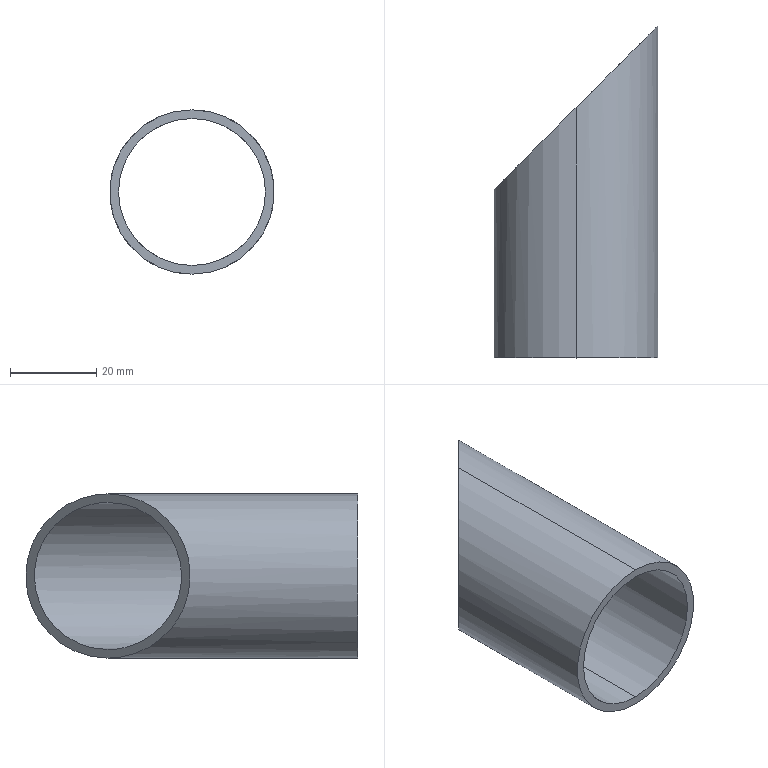Part | SolidWorks | features Extrusion 1, ICE 1 | 1 solid | 6 faces | box 38.1 x 77 x 38.1 mm | volume 13144 mm3 | cylinder 4 | plane 2 | commonest cylinder face diameters 34.1 x2 38.1 x2
STEP:
#1=CARTESIAN_POINT('',(0.,57.95,17.05));
#2=VERTEX_POINT('',#1);
#3=CARTESIAN_POINT('',(0.,57.95,-17.05));
#4=VERTEX_POINT('',#3);
#5=CARTESIAN_POINT('',(0.,57.95,17.05));
#6=CARTESIAN_POINT('',(-34.1,23.85,17.05));
#7=CARTESIAN_POINT('',(-34.1,23.85,-17.05));
#8=CARTESIAN_POINT('',(0.,57.95,-17.05));
#9=(BOUNDED_CURVE()B_SPLINE_CURVE(3,(#5,#6,#7,#8),.UNSPECIFIED.,.F.,.F.)B_SPLINE_CURVE_WITH_KNOTS((4,4),(4.712,7.854),.UNSPECIFIED.)CURVE()GEOMETRIC_REPRESENTATION_ITEM()RATIONAL_B_SPLINE_CURVE((1.,0.3333,0.3333,1.))REPRESENTATION_ITEM(''));
#10=EDGE_CURVE('',#2,#4,#9,.T.);
#11=ORIENTED_EDGE('',*,*,#10,.F.);
#12=CARTESIAN_POINT('',(0.,0.,17.05));
#13=VERTEX_POINT('',#12);
#14=CARTESIAN_POINT('',(0.,77.,17.05));
#15=DIRECTION('',(0.,-1.,0.));
#16=VECTOR('',#15,1000.);
#17=LINE('',#14,#16);
#18=EDGE_CURVE('',#2,#13,#17,.T.);
#19=ORIENTED_EDGE('',*,*,#18,.T.);
#20=CARTESIAN_POINT('',(0.,0.,-17.05));
#21=VERTEX_POINT('',#20);
#22=CARTESIAN_POINT('',(0.,0.,0.));
#23=DIRECTION('',(0.,1.,0.));
#24=DIRECTION('',(0.,0.,1.));
#25=AXIS2_PLACEMENT_3D('',#22,#23,#24);
#26=CIRCLE('',#25,17.05);
#27=EDGE_CURVE('',#21,#13,#26,.T.);
#28=ORIENTED_EDGE('',*,*,#27,.F.);
#29=CARTESIAN_POINT('',(0.,77.,-17.05));
#30=DIRECTION('',(0.,-1.,0.));
#31=VECTOR('',#30,1000.);
#32=LINE('',#29,#31);
#33=EDGE_CURVE('',#4,#21,#32,.T.);
#34=ORIENTED_EDGE('',*,*,#33,.F.);
#35=EDGE_LOOP('',(#11,#19,#28,#34));
#36=FACE_OUTER_BOUND('',#35,.T.);
#37=CARTESIAN_POINT('',(0.,77.,0.));
#38=DIRECTION('',(0.,-1.,0.));
#39=DIRECTION('',(0.,0.,-1.));
#40=AXIS2_PLACEMENT_3D('',#37,#38,#39);
#41=CYLINDRICAL_SURFACE('',#40,17.05);
#42=ADVANCED_FACE('',(#36),#41,.F.);
#43=CARTESIAN_POINT('',(0.,57.95,-19.05));
#44=VERTEX_POINT('',#43);
#45=CARTESIAN_POINT('',(0.,57.95,19.05));
#46=VERTEX_POINT('',#45);
#47=CARTESIAN_POINT('',(0.,57.95,-19.05));
#48=CARTESIAN_POINT('',(38.1,96.05,-19.05));
#49=CARTESIAN_POINT('',(38.1,96.05,19.05));
#50=CARTESIAN_POINT('',(0.,57.95,19.05));
#51=(BOUNDED_CURVE()B_SPLINE_CURVE(3,(#47,#48,#49,#50),.UNSPECIFIED.,.F.,.T.)B_SPLINE_CURVE_WITH_KNOTS((4,4),(1.571,4.712),.UNSPECIFIED.)CURVE()GEOMETRIC_REPRESENTATION_ITEM()RATIONAL_B_SPLINE_CURVE((1.,0.3333,0.3333,1.))REPRESENTATION_ITEM(''));
#52=EDGE_CURVE('',#44,#46,#51,.T.);
#53=ORIENTED_EDGE('',*,*,#52,.T.);
#54=CARTESIAN_POINT('',(0.,0.,19.05));
#55=VERTEX_POINT('',#54);
#56=CARTESIAN_POINT('',(0.,77.,19.05));
#57=DIRECTION('',(0.,-1.,0.));
#58=VECTOR('',#57,1000.);
#59=LINE('',#56,#58);
#60=EDGE_CURVE('',#46,#55,#59,.T.);
#61=ORIENTED_EDGE('',*,*,#60,.T.);
#62=CARTESIAN_POINT('',(0.,0.,-19.05));
#63=VERTEX_POINT('',#62);
#64=CARTESIAN_POINT('',(0.,0.,0.));
#65=DIRECTION('',(0.,1.,0.));
#66=DIRECTION('',(0.,0.,1.));
#67=AXIS2_PLACEMENT_3D('',#64,#65,#66);
#68=CIRCLE('',#67,19.05);
#69=EDGE_CURVE('',#55,#63,#68,.T.);
#70=ORIENTED_EDGE('',*,*,#69,.T.);
#71=CARTESIAN_POINT('',(0.,77.,-19.05));
#72=DIRECTION('',(0.,-1.,0.));
#73=VECTOR('',#72,1000.);
#74=LINE('',#71,#73);
#75=EDGE_CURVE('',#44,#63,#74,.T.);
#76=ORIENTED_EDGE('',*,*,#75,.F.);
#77=EDGE_LOOP('',(#53,#61,#70,#76));
#78=FACE_OUTER_BOUND('',#77,.T.);
#79=CARTESIAN_POINT('',(0.,77.,0.));
#80=DIRECTION('',(0.,-1.,0.));
#81=DIRECTION('',(0.,0.,-1.));
#82=AXIS2_PLACEMENT_3D('',#79,#80,#81);
#83=CYLINDRICAL_SURFACE('',#82,19.05);
#84=ADVANCED_FACE('',(#78),#83,.T.);
#85=ORIENTED_EDGE('',*,*,#60,.F.);
#86=CARTESIAN_POINT('',(0.,57.95,19.05));
#87=CARTESIAN_POINT('',(-38.1,19.85,19.05));
#88=CARTESIAN_POINT('',(-38.1,19.85,-19.05));
#89=CARTESIAN_POINT('',(0.,57.95,-19.05));
#90=(BOUNDED_CURVE()B_SPLINE_CURVE(3,(#86,#87,#88,#89),.UNSPECIFIED.,.F.,.T.)B_SPLINE_CURVE_WITH_KNOTS((4,4),(4.712,7.854),.UNSPECIFIED.)CURVE()GEOMETRIC_REPRESENTATION_ITEM()RATIONAL_B_SPLINE_CURVE((1.,0.3333,0.3333,1.))REPRESENTATION_ITEM(''));
#91=EDGE_CURVE('',#46,#44,#90,.T.);
#92=ORIENTED_EDGE('',*,*,#91,.T.);
#93=ORIENTED_EDGE('',*,*,#75,.T.);
#94=CARTESIAN_POINT('',(0.,0.,0.));
#95=DIRECTION('',(0.,1.,0.));
#96=DIRECTION('',(0.,0.,1.));
#97=AXIS2_PLACEMENT_3D('',#94,#95,#96);
#98=CIRCLE('',#97,19.05);
#99=EDGE_CURVE('',#63,#55,#98,.T.);
#100=ORIENTED_EDGE('',*,*,#99,.T.);
#101=EDGE_LOOP('',(#85,#92,#93,#100));
#102=FACE_OUTER_BOUND('',#101,.T.);
#103=CARTESIAN_POINT('',(0.,77.,0.));
#104=DIRECTION('',(0.,-1.,0.));
#105=DIRECTION('',(0.,0.,-1.));
#106=AXIS2_PLACEMENT_3D('',#103,#104,#105);
#107=CYLINDRICAL_SURFACE('',#106,19.05);
#108=ADVANCED_FACE('',(#102),#107,.T.);
#109=ORIENTED_EDGE('',*,*,#99,.F.);
#110=ORIENTED_EDGE('',*,*,#69,.F.);
#111=EDGE_LOOP('',(#109,#110));
#112=FACE_OUTER_BOUND('',#111,.T.);
#113=ORIENTED_EDGE('',*,*,#27,.T.);
#114=CARTESIAN_POINT('',(0.,0.,0.));
#115=DIRECTION('',(0.,1.,0.));
#116=DIRECTION('',(0.,0.,1.));
#117=AXIS2_PLACEMENT_3D('',#114,#115,#116);
#118=CIRCLE('',#117,17.05);
#119=EDGE_CURVE('',#13,#21,#118,.T.);
#120=ORIENTED_EDGE('',*,*,#119,.T.);
#121=EDGE_LOOP('',(#113,#120));
#122=FACE_BOUND('',#121,.T.);
#123=CARTESIAN_POINT('',(0.,0.,0.));
#124=DIRECTION('',(0.,1.,0.));
#125=DIRECTION('',(0.,0.,1.));
#126=AXIS2_PLACEMENT_3D('',#123,#124,#125);
#127=PLANE('',#126);
#128=ADVANCED_FACE('',(#112,#122),#127,.F.);
#129=ORIENTED_EDGE('',*,*,#18,.F.);
#130=CARTESIAN_POINT('',(0.,57.95,-17.05));
#131=CARTESIAN_POINT('',(34.1,92.05,-17.05));
#132=CARTESIAN_POINT('',(34.1,92.05,17.05));
#133=CARTESIAN_POINT('',(0.,57.95,17.05));
#134=(BOUNDED_CURVE()B_SPLINE_CURVE(3,(#130,#131,#132,#133),.UNSPECIFIED.,.F.,.F.)B_SPLINE_CURVE_WITH_KNOTS((4,4),(1.571,4.712),.UNSPECIFIED.)CURVE()GEOMETRIC_REPRESENTATION_ITEM()RATIONAL_B_SPLINE_CURVE((1.,0.3333,0.3333,1.))REPRESENTATION_ITEM(''));
#135=EDGE_CURVE('',#4,#2,#134,.T.);
#136=ORIENTED_EDGE('',*,*,#135,.F.);
#137=ORIENTED_EDGE('',*,*,#33,.T.);
#138=ORIENTED_EDGE('',*,*,#119,.F.);
#139=EDGE_LOOP('',(#129,#136,#137,#138));
#140=FACE_OUTER_BOUND('',#139,.T.);
#141=CARTESIAN_POINT('',(0.,77.,0.));
#142=DIRECTION('',(0.,-1.,0.));
#143=DIRECTION('',(0.,0.,-1.));
#144=AXIS2_PLACEMENT_3D('',#141,#142,#143);
#145=CYLINDRICAL_SURFACE('',#144,17.05);
#146=ADVANCED_FACE('',(#140),#145,.F.);
#147=ORIENTED_EDGE('',*,*,#135,.T.);
#148=ORIENTED_EDGE('',*,*,#10,.T.);
#149=EDGE_LOOP('',(#147,#148));
#150=FACE_BOUND('',#149,.T.);
#151=ORIENTED_EDGE('',*,*,#52,.F.);
#152=ORIENTED_EDGE('',*,*,#91,.F.);
#153=EDGE_LOOP('',(#151,#152));
#154=FACE_OUTER_BOUND('',#153,.T.);
#155=CARTESIAN_POINT('',(19.05,77.,-19.05));
#156=DIRECTION('',(0.7071,-0.7071,0.));
#157=DIRECTION('',(0.7071,0.7071,0.));
#158=AXIS2_PLACEMENT_3D('',#155,#156,#157);
#159=PLANE('',#158);
#160=ADVANCED_FACE('',(#150,#154),#159,.F.);
#161=CLOSED_SHELL('',(#42,#84,#108,#128,#146,#160));
#162=MANIFOLD_SOLID_BREP('',#161);
#163=CARTESIAN_POINT('',(0.,0.,0.));
#164=DIRECTION('',(0.,0.,1.));
#165=DIRECTION('',(1.,0.,0.));
#166=AXIS2_PLACEMENT_3D('',#163,#164,#165);
#167=(LENGTH_UNIT()NAMED_UNIT(*)SI_UNIT(.MILLI.,.METRE.));
#168=UNCERTAINTY_MEASURE_WITH_UNIT(LENGTH_MEASURE(0.00001),#167,'','');
#169=(NAMED_UNIT(*)PLANE_ANGLE_UNIT()SI_UNIT($,.RADIAN.));
#170=(NAMED_UNIT(*)SI_UNIT($,.STERADIAN.)SOLID_ANGLE_UNIT());
#171=(GEOMETRIC_REPRESENTATION_CONTEXT(3)GLOBAL_UNCERTAINTY_ASSIGNED_CONTEXT((#168))GLOBAL_UNIT_ASSIGNED_CONTEXT((#167,#169,#170))REPRESENTATION_CONTEXT('',''));
#172=ADVANCED_BREP_SHAPE_REPRESENTATION('',(#162,#166),#171);